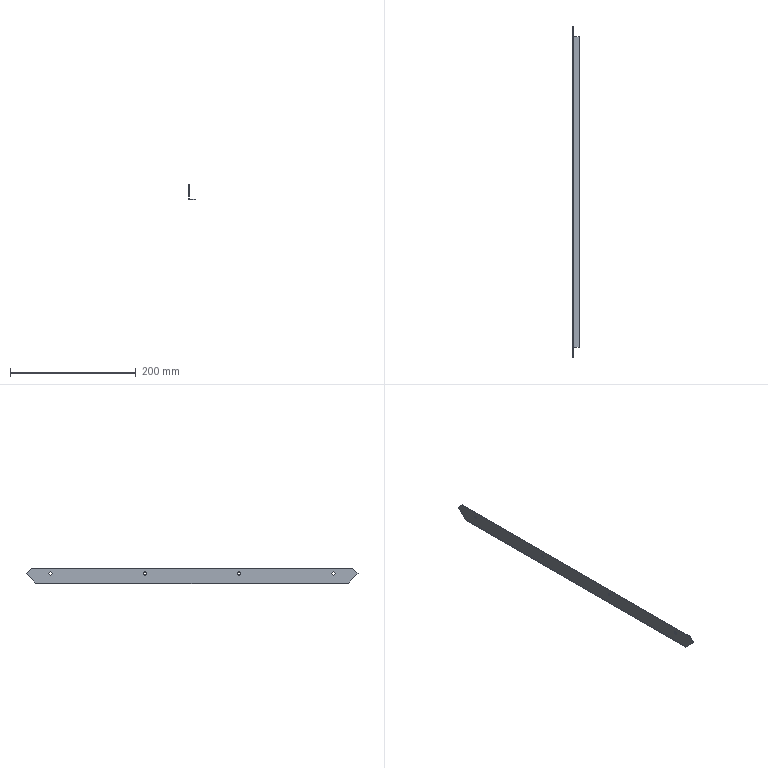Part | STEP file | 1 solid | 24 faces | box 10 x 527.858 x 25 mm | volume 17063 mm3 | plane 12 | cylinder 10 | spline 2 | commonest cylinder face diameters 5 x8 0.4 x1 2.4 x1